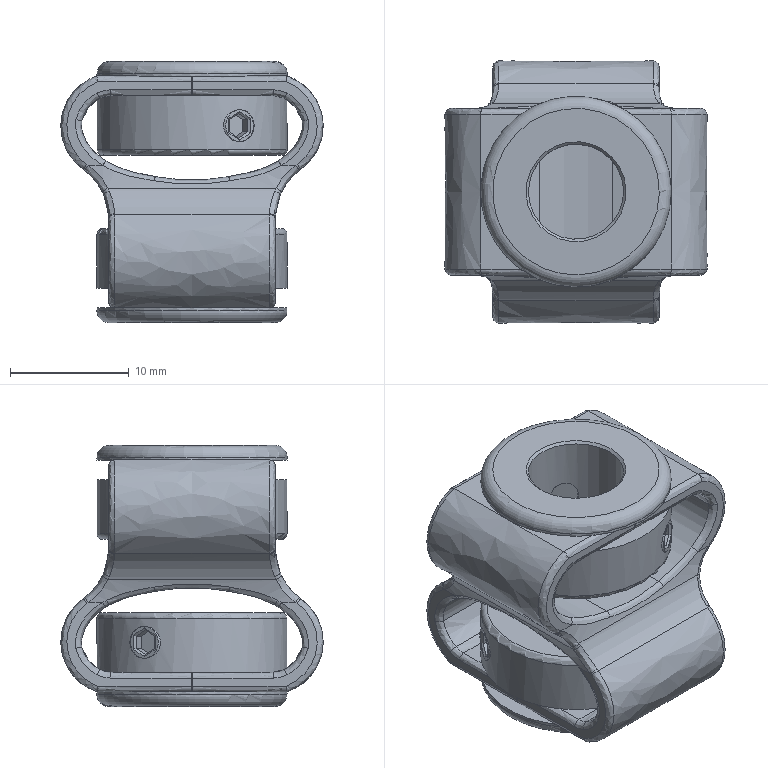Part | NX | features BREP 1 | 1 solid | 254 faces | box 22.041 x 22.041 x 21.943 mm | volume 3971 mm3 | spline 116 | plane 104 | cylinder 18 | cone 12 | torus 4 | commonest cylinder face diameters 2.5 x8 12 x4 16 x4 8 x2